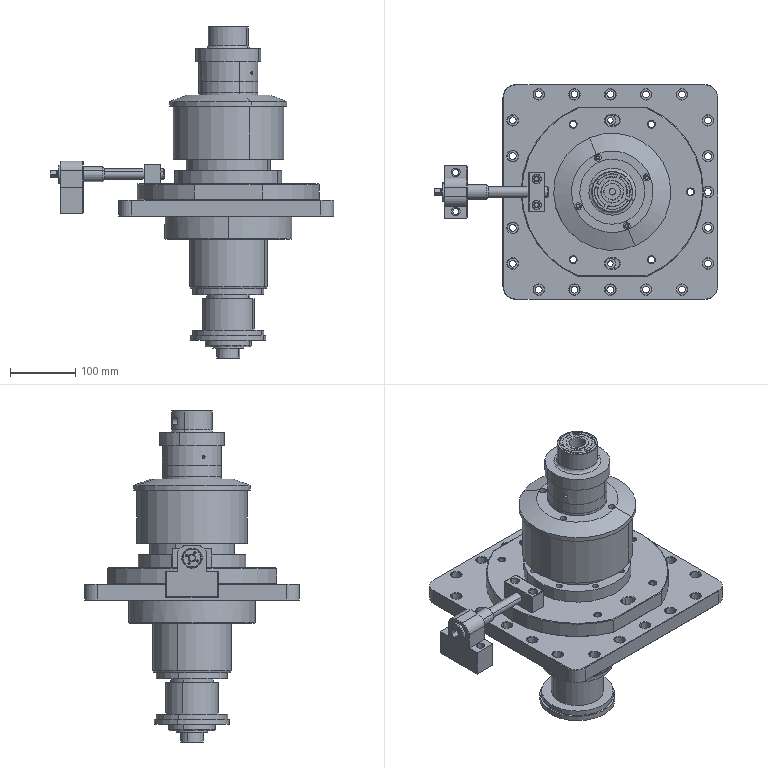Part | SolidWorks | 15 solids | 1075 faces | box 435.5 x 330 x 510 mm | volume 9332980 mm3 | cylinder 397 | cone 348 | plane 288 | spline 42 | commonest cylinder face diameters 10.5 x56 16.5 x40 6.5 x28 9 x24 5 x22 2.5 x16